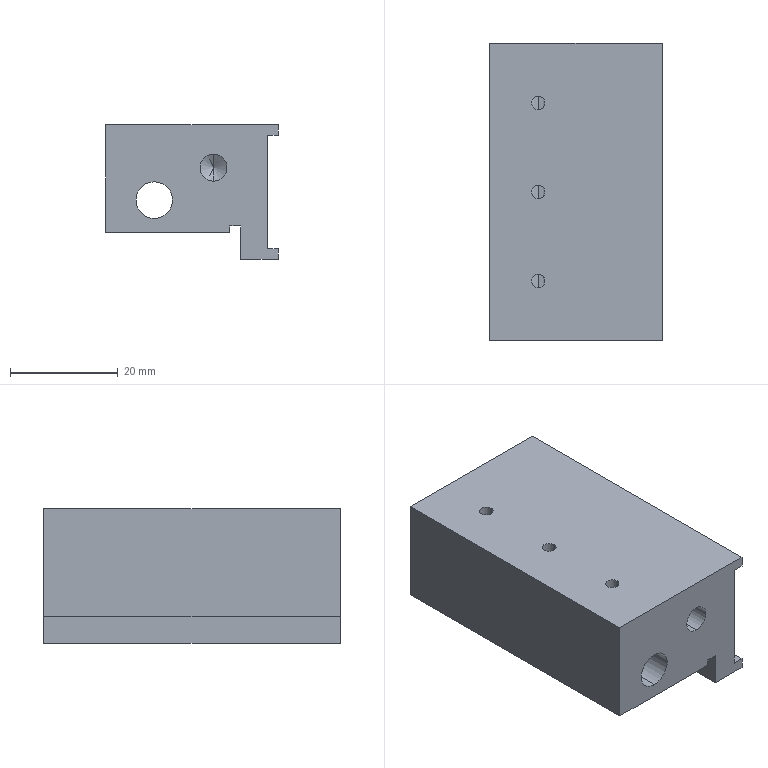Part | STEP file | 11-FG-B03311 | 1 solid | 44 faces | box 32 x 55 x 25 mm | volume 31224 mm3 | cylinder 20 | plane 16 | cone 8 | commonest cylinder face diameters 5 x8 2.5 x6 3.3 x4 6.8 x2
STEP:
#1=CARTESIAN_POINT('',(7.75,27.5,9.162));
#2=VERTEX_POINT('',#1);
#3=CARTESIAN_POINT('',(9.,26.25,9.4));
#4=VERTEX_POINT('',#3);
#5=CARTESIAN_POINT('',(7.75,27.5,9.162));
#6=CARTESIAN_POINT('',(7.75,27.336,9.162));
#7=CARTESIAN_POINT('',(7.783,27.17,9.176));
#8=CARTESIAN_POINT('',(7.909,26.868,9.221));
#9=CARTESIAN_POINT('',(8.001,26.732,9.252));
#10=CARTESIAN_POINT('',(8.232,26.501,9.314));
#11=CARTESIAN_POINT('',(8.368,26.409,9.344));
#12=CARTESIAN_POINT('',(8.595,26.315,9.377));
#13=CARTESIAN_POINT('',(8.673,26.291,9.385));
#14=CARTESIAN_POINT('',(8.834,26.258,9.397));
#15=CARTESIAN_POINT('',(8.918,26.25,9.4));
#16=CARTESIAN_POINT('',(9.,26.25,9.4));
#17=B_SPLINE_CURVE_WITH_KNOTS('',3,(#5,#6,#7,#8,#9,#10,#11,#12,#13,#14,#15,#16),.UNSPECIFIED.,.F.,.F.,(4,2,2,2,2,4),(0.003943,0.004435,0.004928,0.005421,0.005667,0.005913),.UNSPECIFIED.);
#18=EDGE_CURVE('',#2,#4,#17,.T.);
#19=ORIENTED_EDGE('',*,*,#18,.F.);
#20=CARTESIAN_POINT('',(7.75,27.5,20.));
#21=VERTEX_POINT('',#20);
#22=CARTESIAN_POINT('',(7.75,27.5,20.));
#23=DIRECTION('',(0.,0.,1.));
#24=VECTOR('',#23,1000.);
#25=LINE('',#22,#24);
#26=EDGE_CURVE('',#2,#21,#25,.T.);
#27=ORIENTED_EDGE('',*,*,#26,.T.);
#28=CARTESIAN_POINT('',(10.25,27.5,20.));
#29=VERTEX_POINT('',#28);
#30=CARTESIAN_POINT('',(9.,27.5,20.));
#31=DIRECTION('',(0.,0.,1.));
#32=DIRECTION('',(1.,0.,0.));
#33=AXIS2_PLACEMENT_3D('',#30,#31,#32);
#34=CIRCLE('',#33,1.25);
#35=EDGE_CURVE('',#21,#29,#34,.T.);
#36=ORIENTED_EDGE('',*,*,#35,.T.);
#37=CARTESIAN_POINT('',(10.25,27.5,9.162));
#38=VERTEX_POINT('',#37);
#39=CARTESIAN_POINT('',(10.25,27.5,20.));
#40=DIRECTION('',(0.,0.,1.));
#41=VECTOR('',#40,1000.);
#42=LINE('',#39,#41);
#43=EDGE_CURVE('',#38,#29,#42,.T.);
#44=ORIENTED_EDGE('',*,*,#43,.F.);
#45=CARTESIAN_POINT('',(9.,26.25,9.4));
#46=CARTESIAN_POINT('',(9.165,26.25,9.4));
#47=CARTESIAN_POINT('',(9.33,26.283,9.387));
#48=CARTESIAN_POINT('',(9.632,26.409,9.344));
#49=CARTESIAN_POINT('',(9.77,26.502,9.314));
#50=CARTESIAN_POINT('',(9.999,26.731,9.252));
#51=CARTESIAN_POINT('',(10.091,26.868,9.221));
#52=CARTESIAN_POINT('',(10.217,27.171,9.175));
#53=CARTESIAN_POINT('',(10.25,27.333,9.162));
#54=CARTESIAN_POINT('',(10.25,27.5,9.162));
#55=B_SPLINE_CURVE_WITH_KNOTS('',3,(#45,#46,#47,#48,#49,#50,#51,#52,#53,#54),.UNSPECIFIED.,.F.,.F.,(4,2,2,2,4),(0.005913,0.006406,0.006899,0.007392,0.007885),.UNSPECIFIED.);
#56=EDGE_CURVE('',#4,#38,#55,.T.);
#57=ORIENTED_EDGE('',*,*,#56,.F.);
#58=EDGE_LOOP('',(#19,#27,#36,#44,#57));
#59=FACE_OUTER_BOUND('',#58,.T.);
#60=CARTESIAN_POINT('',(9.,27.5,20.));
#61=DIRECTION('',(0.,0.,1.));
#62=DIRECTION('',(1.,0.,0.));
#63=AXIS2_PLACEMENT_3D('',#60,#61,#62);
#64=CYLINDRICAL_SURFACE('',#63,1.25);
#65=ADVANCED_FACE('',(#59),#64,.F.);
#66=CARTESIAN_POINT('',(7.75,44.,9.162));
#67=VERTEX_POINT('',#66);
#68=CARTESIAN_POINT('',(9.,42.75,9.4));
#69=VERTEX_POINT('',#68);
#70=CARTESIAN_POINT('',(7.75,44.,9.162));
#71=CARTESIAN_POINT('',(7.75,43.836,9.162));
#72=CARTESIAN_POINT('',(7.783,43.67,9.176));
#73=CARTESIAN_POINT('',(7.909,43.368,9.221));
#74=CARTESIAN_POINT('',(8.001,43.232,9.252));
#75=CARTESIAN_POINT('',(8.232,43.001,9.314));
#76=CARTESIAN_POINT('',(8.368,42.909,9.344));
#77=CARTESIAN_POINT('',(8.595,42.815,9.377));
#78=CARTESIAN_POINT('',(8.673,42.791,9.385));
#79=CARTESIAN_POINT('',(8.834,42.758,9.397));
#80=CARTESIAN_POINT('',(8.918,42.75,9.4));
#81=CARTESIAN_POINT('',(9.,42.75,9.4));
#82=B_SPLINE_CURVE_WITH_KNOTS('',3,(#70,#71,#72,#73,#74,#75,#76,#77,#78,#79,#80,#81),.UNSPECIFIED.,.F.,.F.,(4,2,2,2,2,4),(0.003943,0.004435,0.004928,0.005421,0.005667,0.005913),.UNSPECIFIED.);
#83=EDGE_CURVE('',#67,#69,#82,.T.);
#84=ORIENTED_EDGE('',*,*,#83,.F.);
#85=CARTESIAN_POINT('',(7.75,44.,20.));
#86=VERTEX_POINT('',#85);
#87=CARTESIAN_POINT('',(7.75,44.,20.));
#88=DIRECTION('',(0.,0.,1.));
#89=VECTOR('',#88,1000.);
#90=LINE('',#87,#89);
#91=EDGE_CURVE('',#67,#86,#90,.T.);
#92=ORIENTED_EDGE('',*,*,#91,.T.);
#93=CARTESIAN_POINT('',(10.25,44.,20.));
#94=VERTEX_POINT('',#93);
#95=CARTESIAN_POINT('',(9.,44.,20.));
#96=DIRECTION('',(0.,0.,1.));
#97=DIRECTION('',(1.,0.,0.));
#98=AXIS2_PLACEMENT_3D('',#95,#96,#97);
#99=CIRCLE('',#98,1.25);
#100=EDGE_CURVE('',#86,#94,#99,.T.);
#101=ORIENTED_EDGE('',*,*,#100,.T.);
#102=CARTESIAN_POINT('',(10.25,44.,9.162));
#103=VERTEX_POINT('',#102);
#104=CARTESIAN_POINT('',(10.25,44.,20.));
#105=DIRECTION('',(0.,0.,1.));
#106=VECTOR('',#105,1000.);
#107=LINE('',#104,#106);
#108=EDGE_CURVE('',#103,#94,#107,.T.);
#109=ORIENTED_EDGE('',*,*,#108,.F.);
#110=CARTESIAN_POINT('',(9.,42.75,9.4));
#111=CARTESIAN_POINT('',(9.165,42.75,9.4));
#112=CARTESIAN_POINT('',(9.33,42.783,9.387));
#113=CARTESIAN_POINT('',(9.632,42.909,9.344));
#114=CARTESIAN_POINT('',(9.77,43.002,9.314));
#115=CARTESIAN_POINT('',(9.999,43.231,9.252));
#116=CARTESIAN_POINT('',(10.091,43.368,9.221));
#117=CARTESIAN_POINT('',(10.217,43.671,9.175));
#118=CARTESIAN_POINT('',(10.25,43.833,9.162));
#119=CARTESIAN_POINT('',(10.25,44.,9.162));
#120=B_SPLINE_CURVE_WITH_KNOTS('',3,(#110,#111,#112,#113,#114,#115,#116,#117,#118,#119),.UNSPECIFIED.,.F.,.F.,(4,2,2,2,4),(0.005913,0.006406,0.006899,0.007392,0.007885),.UNSPECIFIED.);
#121=EDGE_CURVE('',#69,#103,#120,.T.);
#122=ORIENTED_EDGE('',*,*,#121,.F.);
#123=EDGE_LOOP('',(#84,#92,#101,#109,#122));
#124=FACE_OUTER_BOUND('',#123,.T.);
#125=CARTESIAN_POINT('',(9.,44.,20.));
#126=DIRECTION('',(0.,0.,1.));
#127=DIRECTION('',(1.,0.,0.));
#128=AXIS2_PLACEMENT_3D('',#125,#126,#127);
#129=CYLINDRICAL_SURFACE('',#128,1.25);
#130=ADVANCED_FACE('',(#124),#129,.F.);
#131=CARTESIAN_POINT('',(7.75,11.,9.162));
#132=VERTEX_POINT('',#131);
#133=CARTESIAN_POINT('',(9.,9.75,9.4));
#134=VERTEX_POINT('',#133);
#135=CARTESIAN_POINT('',(7.75,11.,9.162));
#136=CARTESIAN_POINT('',(7.75,10.836,9.162));
#137=CARTESIAN_POINT('',(7.783,10.67,9.176));
#138=CARTESIAN_POINT('',(7.909,10.368,9.221));
#139=CARTESIAN_POINT('',(8.001,10.232,9.252));
#140=CARTESIAN_POINT('',(8.232,10.001,9.314));
#141=CARTESIAN_POINT('',(8.368,9.909,9.344));
#142=CARTESIAN_POINT('',(8.595,9.815,9.377));
#143=CARTESIAN_POINT('',(8.673,9.791,9.385));
#144=CARTESIAN_POINT('',(8.834,9.758,9.397));
#145=CARTESIAN_POINT('',(8.918,9.75,9.4));
#146=CARTESIAN_POINT('',(9.,9.75,9.4));
#147=B_SPLINE_CURVE_WITH_KNOTS('',3,(#135,#136,#137,#138,#139,#140,#141,#142,#143,#144,#145,#146),.UNSPECIFIED.,.F.,.F.,(4,2,2,2,2,4),(0.003943,0.004435,0.004928,0.005421,0.005667,0.005913),.UNSPECIFIED.);
#148=EDGE_CURVE('',#132,#134,#147,.T.);
#149=ORIENTED_EDGE('',*,*,#148,.F.);
#150=CARTESIAN_POINT('',(7.75,11.,20.));
#151=VERTEX_POINT('',#150);
#152=CARTESIAN_POINT('',(7.75,11.,20.));
#153=DIRECTION('',(0.,0.,1.));
#154=VECTOR('',#153,1000.);
#155=LINE('',#152,#154);
#156=EDGE_CURVE('',#132,#151,#155,.T.);
#157=ORIENTED_EDGE('',*,*,#156,.T.);
#158=CARTESIAN_POINT('',(10.25,11.,20.));
#159=VERTEX_POINT('',#158);
#160=CARTESIAN_POINT('',(9.,11.,20.));
#161=DIRECTION('',(0.,0.,1.));
#162=DIRECTION('',(1.,0.,0.));
#163=AXIS2_PLACEMENT_3D('',#160,#161,#162);
#164=CIRCLE('',#163,1.25);
#165=EDGE_CURVE('',#151,#159,#164,.T.);
#166=ORIENTED_EDGE('',*,*,#165,.T.);
#167=CARTESIAN_POINT('',(10.25,11.,9.162));
#168=VERTEX_POINT('',#167);
#169=CARTESIAN_POINT('',(10.25,11.,20.));
#170=DIRECTION('',(0.,0.,1.));
#171=VECTOR('',#170,1000.);
#172=LINE('',#169,#171);
#173=EDGE_CURVE('',#168,#159,#172,.T.);
#174=ORIENTED_EDGE('',*,*,#173,.F.);
#175=CARTESIAN_POINT('',(9.,9.75,9.4));
#176=CARTESIAN_POINT('',(9.165,9.75,9.4));
#177=CARTESIAN_POINT('',(9.33,9.783,9.387));
#178=CARTESIAN_POINT('',(9.632,9.909,9.344));
#179=CARTESIAN_POINT('',(9.77,10.002,9.314));
#180=CARTESIAN_POINT('',(9.999,10.231,9.252));
#181=CARTESIAN_POINT('',(10.091,10.368,9.221));
#182=CARTESIAN_POINT('',(10.217,10.671,9.175));
#183=CARTESIAN_POINT('',(10.25,10.833,9.162));
#184=CARTESIAN_POINT('',(10.25,11.,9.162));
#185=B_SPLINE_CURVE_WITH_KNOTS('',3,(#175,#176,#177,#178,#179,#180,#181,#182,#183,#184),.UNSPECIFIED.,.F.,.F.,(4,2,2,2,4),(0.005913,0.006406,0.006899,0.007392,0.007885),.UNSPECIFIED.);
#186=EDGE_CURVE('',#134,#168,#185,.T.);
#187=ORIENTED_EDGE('',*,*,#186,.F.);
#188=EDGE_LOOP('',(#149,#157,#166,#174,#187));
#189=FACE_OUTER_BOUND('',#188,.T.);
#190=CARTESIAN_POINT('',(9.,11.,20.));
#191=DIRECTION('',(0.,0.,1.));
#192=DIRECTION('',(1.,0.,0.));
#193=AXIS2_PLACEMENT_3D('',#190,#191,#192);
#194=CYLINDRICAL_SURFACE('',#193,1.25);
#195=ADVANCED_FACE('',(#189),#194,.F.);
#196=CARTESIAN_POINT('',(20.,40.,9.5));
#197=VERTEX_POINT('',#196);
#198=CARTESIAN_POINT('',(20.,40.,14.5));
#199=VERTEX_POINT('',#198);
#200=CARTESIAN_POINT('',(20.,40.,12.));
#201=DIRECTION('',(0.,1.,0.));
#202=DIRECTION('',(0.,0.,1.));
#203=AXIS2_PLACEMENT_3D('',#200,#201,#202);
#204=CIRCLE('',#203,2.5);
#205=EDGE_CURVE('',#197,#199,#204,.T.);
#206=ORIENTED_EDGE('',*,*,#205,.F.);
#207=CARTESIAN_POINT('',(20.,55.,9.5));
#208=VERTEX_POINT('',#207);
#209=CARTESIAN_POINT('',(20.,55.,9.5));
#210=DIRECTION('',(0.,1.,0.));
#211=VECTOR('',#210,1000.);
#212=LINE('',#209,#211);
#213=EDGE_CURVE('',#197,#208,#212,.T.);
#214=ORIENTED_EDGE('',*,*,#213,.T.);
#215=CARTESIAN_POINT('',(20.,55.,14.5));
#216=VERTEX_POINT('',#215);
#217=CARTESIAN_POINT('',(20.,55.,12.));
#218=DIRECTION('',(0.,1.,0.));
#219=DIRECTION('',(0.,0.,1.));
#220=AXIS2_PLACEMENT_3D('',#217,#218,#219);
#221=CIRCLE('',#220,2.5);
#222=EDGE_CURVE('',#208,#216,#221,.T.);
#223=ORIENTED_EDGE('',*,*,#222,.T.);
#224=CARTESIAN_POINT('',(20.,55.,14.5));
#225=DIRECTION('',(0.,1.,0.));
#226=VECTOR('',#225,1000.);
#227=LINE('',#224,#226);
#228=EDGE_CURVE('',#199,#216,#227,.T.);
#229=ORIENTED_EDGE('',*,*,#228,.F.);
#230=EDGE_LOOP('',(#206,#214,#223,#229));
#231=FACE_OUTER_BOUND('',#230,.T.);
#232=CARTESIAN_POINT('',(20.,55.,12.));
#233=DIRECTION('',(0.,1.,0.));
#234=DIRECTION('',(0.,0.,1.));
#235=AXIS2_PLACEMENT_3D('',#232,#233,#234);
#236=CYLINDRICAL_SURFACE('',#235,2.5);
#237=ADVANCED_FACE('',(#231),#236,.F.);
#238=CARTESIAN_POINT('',(20.,38.498,12.));
#239=VERTEX_POINT('',#238);
#240=CARTESIAN_POINT('',(20.,40.,14.5));
#241=DIRECTION('',(0.,0.515,0.8572));
#242=VECTOR('',#241,1000.);
#243=LINE('',#240,#242);
#244=EDGE_CURVE('',#239,#199,#243,.T.);
#245=ORIENTED_EDGE('',*,*,#244,.F.);
#246=CARTESIAN_POINT('',(20.,40.,9.5));
#247=DIRECTION('',(0.,0.515,-0.8572));
#248=VECTOR('',#247,1000.);
#249=LINE('',#246,#248);
#250=EDGE_CURVE('',#239,#197,#249,.T.);
#251=ORIENTED_EDGE('',*,*,#250,.T.);
#252=ORIENTED_EDGE('',*,*,#205,.T.);
#253=EDGE_LOOP('',(#245,#251,#252));
#254=FACE_OUTER_BOUND('',#253,.T.);
#255=CARTESIAN_POINT('',(20.,40.,12.));
#256=DIRECTION('',(0.,1.,0.));
#257=DIRECTION('',(0.,0.,1.));
#258=AXIS2_PLACEMENT_3D('',#255,#256,#257);
#259=CONICAL_SURFACE('',#258,2.5,1.03);
#260=ADVANCED_FACE('',(#254),#259,.F.);
#261=CARTESIAN_POINT('',(18.,48.5,9.));
#262=VERTEX_POINT('',#261);
#263=CARTESIAN_POINT('',(18.,48.5,4.));
#264=VERTEX_POINT('',#263);
#265=CARTESIAN_POINT('',(18.,48.5,6.5));
#266=DIRECTION('',(1.,0.,0.));
#267=DIRECTION('',(0.,0.,-1.));
#268=AXIS2_PLACEMENT_3D('',#265,#266,#267);
#269=CIRCLE('',#268,2.5);
#270=EDGE_CURVE('',#262,#264,#269,.T.);
#271=ORIENTED_EDGE('',*,*,#270,.F.);
#272=CARTESIAN_POINT('',(30.,48.5,9.));
#273=VERTEX_POINT('',#272);
#274=CARTESIAN_POINT('',(30.,48.5,9.));
#275=DIRECTION('',(1.,0.,0.));
#276=VECTOR('',#275,1000.);
#277=LINE('',#274,#276);
#278=EDGE_CURVE('',#262,#273,#277,.T.);
#279=ORIENTED_EDGE('',*,*,#278,.T.);
#280=CARTESIAN_POINT('',(30.,48.5,4.));
#281=VERTEX_POINT('',#280);
#282=CARTESIAN_POINT('',(30.,48.5,6.5));
#283=DIRECTION('',(1.,0.,0.));
#284=DIRECTION('',(0.,0.,-1.));
#285=AXIS2_PLACEMENT_3D('',#282,#283,#284);
#286=CIRCLE('',#285,2.5);
#287=EDGE_CURVE('',#273,#281,#286,.T.);
#288=ORIENTED_EDGE('',*,*,#287,.T.);
#289=CARTESIAN_POINT('',(30.,48.5,4.));
#290=DIRECTION('',(1.,0.,0.));
#291=VECTOR('',#290,1000.);
#292=LINE('',#289,#291);
#293=EDGE_CURVE('',#264,#281,#292,.T.);
#294=ORIENTED_EDGE('',*,*,#293,.F.);
#295=EDGE_LOOP('',(#271,#279,#288,#294));
#296=FACE_OUTER_BOUND('',#295,.T.);
#297=CARTESIAN_POINT('',(30.,48.5,6.5));
#298=DIRECTION('',(1.,0.,0.));
#299=DIRECTION('',(0.,0.,-1.));
#300=AXIS2_PLACEMENT_3D('',#297,#298,#299);
#301=CYLINDRICAL_SURFACE('',#300,2.5);
#302=ADVANCED_FACE('',(#296),#301,.F.);
#303=CARTESIAN_POINT('',(16.498,48.5,6.5));
#304=VERTEX_POINT('',#303);
#305=CARTESIAN_POINT('',(18.,48.5,4.));
#306=DIRECTION('',(0.515,0.,-0.8572));
#307=VECTOR('',#306,1000.);
#308=LINE('',#305,#307);
#309=EDGE_CURVE('',#304,#264,#308,.T.);
#310=ORIENTED_EDGE('',*,*,#309,.F.);
#311=CARTESIAN_POINT('',(18.,48.5,9.));
#312=DIRECTION('',(0.515,0.,0.8572));
#313=VECTOR('',#312,1000.);
#314=LINE('',#311,#313);
#315=EDGE_CURVE('',#304,#262,#314,.T.);
#316=ORIENTED_EDGE('',*,*,#315,.T.);
#317=ORIENTED_EDGE('',*,*,#270,.T.);
#318=EDGE_LOOP('',(#310,#316,#317));
#319=FACE_OUTER_BOUND('',#318,.T.);
#320=CARTESIAN_POINT('',(18.,48.5,6.5));
#321=DIRECTION('',(1.,0.,0.));
#322=DIRECTION('',(0.,0.,-1.));
#323=AXIS2_PLACEMENT_3D('',#320,#321,#322);
#324=CONICAL_SURFACE('',#323,2.5,1.03);
#325=ADVANCED_FACE('',(#319),#324,.F.);
#326=CARTESIAN_POINT('',(18.,6.5,9.));
#327=VERTEX_POINT('',#326);
#328=CARTESIAN_POINT('',(18.,6.5,4.));
#329=VERTEX_POINT('',#328);
#330=CARTESIAN_POINT('',(18.,6.5,6.5));
#331=DIRECTION('',(1.,0.,0.));
#332=DIRECTION('',(0.,0.,-1.));
#333=AXIS2_PLACEMENT_3D('',#330,#331,#332);
#334=CIRCLE('',#333,2.5);
#335=EDGE_CURVE('',#327,#329,#334,.T.);
#336=ORIENTED_EDGE('',*,*,#335,.F.);
#337=CARTESIAN_POINT('',(30.,6.5,9.));
#338=VERTEX_POINT('',#337);
#339=CARTESIAN_POINT('',(30.,6.5,9.));
#340=DIRECTION('',(1.,0.,0.));
#341=VECTOR('',#340,1000.);
#342=LINE('',#339,#341);
#343=EDGE_CURVE('',#327,#338,#342,.T.);
#344=ORIENTED_EDGE('',*,*,#343,.T.);
#345=CARTESIAN_POINT('',(30.,6.5,4.));
#346=VERTEX_POINT('',#345);
#347=CARTESIAN_POINT('',(30.,6.5,6.5));
#348=DIRECTION('',(1.,0.,0.));
#349=DIRECTION('',(0.,0.,-1.));
#350=AXIS2_PLACEMENT_3D('',#347,#348,#349);
#351=CIRCLE('',#350,2.5);
#352=EDGE_CURVE('',#338,#346,#351,.T.);
#353=ORIENTED_EDGE('',*,*,#352,.T.);
#354=CARTESIAN_POINT('',(30.,6.5,4.));
#355=DIRECTION('',(1.,0.,0.));
#356=VECTOR('',#355,1000.);
#357=LINE('',#354,#356);
#358=EDGE_CURVE('',#329,#346,#357,.T.);
#359=ORIENTED_EDGE('',*,*,#358,.F.);
#360=EDGE_LOOP('',(#336,#344,#353,#359));
#361=FACE_OUTER_BOUND('',#360,.T.);
#362=CARTESIAN_POINT('',(30.,6.5,6.5));
#363=DIRECTION('',(1.,0.,0.));
#364=DIRECTION('',(0.,0.,-1.));
#365=AXIS2_PLACEMENT_3D('',#362,#363,#364);
#366=CYLINDRICAL_SURFACE('',#365,2.5);
#367=ADVANCED_FACE('',(#361),#366,.F.);
#368=CARTESIAN_POINT('',(16.498,6.5,6.5));
#369=VERTEX_POINT('',#368);
#370=CARTESIAN_POINT('',(18.,6.5,4.));
#371=DIRECTION('',(0.515,0.,-0.8572));
#372=VECTOR('',#371,1000.);
#373=LINE('',#370,#372);
#374=EDGE_CURVE('',#369,#329,#373,.T.);
#375=ORIENTED_EDGE('',*,*,#374,.F.);
#376=CARTESIAN_POINT('',(18.,6.5,9.));
#377=DIRECTION('',(0.515,0.,0.8572));
#378=VECTOR('',#377,1000.);
#379=LINE('',#376,#378);
#380=EDGE_CURVE('',#369,#327,#379,.T.);
#381=ORIENTED_EDGE('',*,*,#380,.T.);
#382=ORIENTED_EDGE('',*,*,#335,.T.);
#383=EDGE_LOOP('',(#375,#381,#382));
#384=FACE_OUTER_BOUND('',#383,.T.);
#385=CARTESIAN_POINT('',(18.,6.5,6.5));
#386=DIRECTION('',(1.,0.,0.));
#387=DIRECTION('',(0.,0.,-1.));
#388=AXIS2_PLACEMENT_3D('',#385,#386,#387);
#389=CONICAL_SURFACE('',#388,2.5,1.03);
#390=ADVANCED_FACE('',(#384),#389,.F.);
#391=CARTESIAN_POINT('',(20.,15.,14.5));
#392=VERTEX_POINT('',#391);
#393=CARTESIAN_POINT('',(20.,15.,9.5));
#394=VERTEX_POINT('',#393);
#395=CARTESIAN_POINT('',(20.,15.,12.));
#396=DIRECTION('',(0.,-1.,0.));
#397=DIRECTION('',(0.,0.,-1.));
#398=AXIS2_PLACEMENT_3D('',#395,#396,#397);
#399=CIRCLE('',#398,2.5);
#400=EDGE_CURVE('',#392,#394,#399,.T.);
#401=ORIENTED_EDGE('',*,*,#400,.F.);
#402=CARTESIAN_POINT('',(20.,0.,14.5));
#403=VERTEX_POINT('',#402);
#404=CARTESIAN_POINT('',(20.,0.,14.5));
#405=DIRECTION('',(0.,-1.,0.));
#406=VECTOR('',#405,1000.);
#407=LINE('',#404,#406);
#408=EDGE_CURVE('',#392,#403,#407,.T.);
#409=ORIENTED_EDGE('',*,*,#408,.T.);
#410=CARTESIAN_POINT('',(20.,0.,9.5));
#411=VERTEX_POINT('',#410);
#412=CARTESIAN_POINT('',(20.,0.,12.));
#413=DIRECTION('',(0.,-1.,0.));
#414=DIRECTION('',(0.,0.,-1.));
#415=AXIS2_PLACEMENT_3D('',#412,#413,#414);
#416=CIRCLE('',#415,2.5);
#417=EDGE_CURVE('',#403,#411,#416,.T.);
#418=ORIENTED_EDGE('',*,*,#417,.T.);
#419=CARTESIAN_POINT('',(20.,0.,9.5));
#420=DIRECTION('',(0.,-1.,0.));
#421=VECTOR('',#420,1000.);
#422=LINE('',#419,#421);
#423=EDGE_CURVE('',#394,#411,#422,.T.);
#424=ORIENTED_EDGE('',*,*,#423,.F.);
#425=EDGE_LOOP('',(#401,#409,#418,#424));
#426=FACE_OUTER_BOUND('',#425,.T.);
#427=CARTESIAN_POINT('',(20.,0.,12.));
#428=DIRECTION('',(0.,-1.,0.));
#429=DIRECTION('',(0.,0.,-1.));
#430=AXIS2_PLACEMENT_3D('',#427,#428,#429);
#431=CYLINDRICAL_SURFACE('',#430,2.5);
#432=ADVANCED_FACE('',(#426),#431,.F.);
#433=CARTESIAN_POINT('',(20.,16.502,12.));
#434=VERTEX_POINT('',#433);
#435=CARTESIAN_POINT('',(20.,15.,9.5));
#436=DIRECTION('',(0.,-0.515,-0.8572));
#437=VECTOR('',#436,1000.);
#438=LINE('',#435,#437);
#439=EDGE_CURVE('',#434,#394,#438,.T.);
#440=ORIENTED_EDGE('',*,*,#439,.F.);
#441=CARTESIAN_POINT('',(20.,15.,14.5));
#442=DIRECTION('',(0.,-0.515,0.8572));
#443=VECTOR('',#442,1000.);
#444=LINE('',#441,#443);
#445=EDGE_CURVE('',#434,#392,#444,.T.);
#446=ORIENTED_EDGE('',*,*,#445,.T.);
#447=ORIENTED_EDGE('',*,*,#400,.T.);
#448=EDGE_LOOP('',(#440,#446,#447));
#449=FACE_OUTER_BOUND('',#448,.T.);
#450=CARTESIAN_POINT('',(20.,15.,12.));
#451=DIRECTION('',(0.,-1.,0.));
#452=DIRECTION('',(0.,0.,-1.));
#453=AXIS2_PLACEMENT_3D('',#450,#451,#452);
#454=CONICAL_SURFACE('',#453,2.5,1.03);
#455=ADVANCED_FACE('',(#449),#454,.F.);
#456=CARTESIAN_POINT('',(16.65,45.,12.));
#457=VERTEX_POINT('',#456);
#458=CARTESIAN_POINT('',(13.35,45.,12.));
#459=VERTEX_POINT('',#458);
#460=CARTESIAN_POINT('',(15.,45.,12.));
#461=DIRECTION('',(0.,0.,-1.));
#462=DIRECTION('',(-1.,0.,0.));
#463=AXIS2_PLACEMENT_3D('',#460,#461,#462);
#464=CIRCLE('',#463,1.65);
#465=EDGE_CURVE('',#457,#459,#464,.T.);
#466=ORIENTED_EDGE('',*,*,#465,.F.);
#467=CARTESIAN_POINT('',(16.65,45.,0.));
#468=VERTEX_POINT('',#467);
#469=CARTESIAN_POINT('',(16.65,45.,0.));
#470=DIRECTION('',(0.,0.,-1.));
#471=VECTOR('',#470,1000.);
#472=LINE('',#469,#471);
#473=EDGE_CURVE('',#457,#468,#472,.T.);
#474=ORIENTED_EDGE('',*,*,#473,.T.);
#475=CARTESIAN_POINT('',(13.35,45.,0.));
#476=VERTEX_POINT('',#475);
#477=CARTESIAN_POINT('',(15.,45.,0.));
#478=DIRECTION('',(0.,0.,-1.));
#479=DIRECTION('',(-1.,0.,0.));
#480=AXIS2_PLACEMENT_3D('',#477,#478,#479);
#481=CIRCLE('',#480,1.65);
#482=EDGE_CURVE('',#468,#476,#481,.T.);
#483=ORIENTED_EDGE('',*,*,#482,.T.);
#484=CARTESIAN_POINT('',(13.35,45.,0.));
#485=DIRECTION('',(0.,0.,-1.));
#486=VECTOR('',#485,1000.);
#487=LINE('',#484,#486);
#488=EDGE_CURVE('',#459,#476,#487,.T.);
#489=ORIENTED_EDGE('',*,*,#488,.F.);
#490=EDGE_LOOP('',(#466,#474,#483,#489));
#491=FACE_OUTER_BOUND('',#490,.T.);
#492=CARTESIAN_POINT('',(15.,45.,0.));
#493=DIRECTION('',(0.,0.,-1.));
#494=DIRECTION('',(-1.,0.,0.));
#495=AXIS2_PLACEMENT_3D('',#492,#493,#494);
#496=CYLINDRICAL_SURFACE('',#495,1.65);
#497=ADVANCED_FACE('',(#491),#496,.F.);
#498=CARTESIAN_POINT('',(16.65,10.,12.));
#499=VERTEX_POINT('',#498);
#500=CARTESIAN_POINT('',(13.35,10.,12.));
#501=VERTEX_POINT('',#500);
#502=CARTESIAN_POINT('',(15.,10.,12.));
#503=DIRECTION('',(0.,0.,-1.));
#504=DIRECTION('',(-1.,0.,0.));
#505=AXIS2_PLACEMENT_3D('',#502,#503,#504);
#506=CIRCLE('',#505,1.65);
#507=EDGE_CURVE('',#499,#501,#506,.T.);
#508=ORIENTED_EDGE('',*,*,#507,.F.);
#509=CARTESIAN_POINT('',(16.65,10.,0.));
#510=VERTEX_POINT('',#509);
#511=CARTESIAN_POINT('',(16.65,10.,0.));
#512=DIRECTION('',(0.,0.,-1.));
#513=VECTOR('',#512,1000.);
#514=LINE('',#511,#513);
#515=EDGE_CURVE('',#499,#510,#514,.T.);
#516=ORIENTED_EDGE('',*,*,#515,.T.);
#517=CARTESIAN_POINT('',(13.35,10.,0.));
#518=VERTEX_POINT('',#517);
#519=CARTESIAN_POINT('',(15.,10.,0.));
#520=DIRECTION('',(0.,0.,-1.));
#521=DIRECTION('',(-1.,0.,0.));
#522=AXIS2_PLACEMENT_3D('',#519,#520,#521);
#523=CIRCLE('',#522,1.65);
#524=EDGE_CURVE('',#510,#518,#523,.T.);
#525=ORIENTED_EDGE('',*,*,#524,.T.);
#526=CARTESIAN_POINT('',(13.35,10.,0.));
#527=DIRECTION('',(0.,0.,-1.));
#528=VECTOR('',#527,1000.);
#529=LINE('',#526,#528);
#530=EDGE_CURVE('',#501,#518,#529,.T.);
#531=ORIENTED_EDGE('',*,*,#530,.F.);
#532=EDGE_LOOP('',(#508,#516,#525,#531));
#533=FACE_OUTER_BOUND('',#532,.T.);
#534=CARTESIAN_POINT('',(15.,10.,0.));
#535=DIRECTION('',(0.,0.,-1.));
#536=DIRECTION('',(-1.,0.,0.));
#537=AXIS2_PLACEMENT_3D('',#534,#535,#536);
#538=CYLINDRICAL_SURFACE('',#537,1.65);
#539=ADVANCED_FACE('',(#533),#538,.F.);
#540=CARTESIAN_POINT('',(9.,55.,9.4));
#541=VERTEX_POINT('',#540);
#542=CARTESIAN_POINT('',(9.,55.,2.6));
#543=VERTEX_POINT('',#542);
#544=CARTESIAN_POINT('',(9.,55.,6.));
#545=DIRECTION('',(0.,-1.,0.));
#546=DIRECTION('',(0.,0.,-1.));
#547=AXIS2_PLACEMENT_3D('',#544,#545,#546);
#548=CIRCLE('',#547,3.4);
#549=EDGE_CURVE('',#541,#543,#548,.T.);
#550=ORIENTED_EDGE('',*,*,#549,.F.);
#551=CARTESIAN_POINT('',(9.,45.25,9.4));
#552=VERTEX_POINT('',#551);
#553=CARTESIAN_POINT('',(9.,55.,9.4));
#554=DIRECTION('',(0.,-1.,0.));
#555=VECTOR('',#554,1000.);
#556=LINE('',#553,#555);
#557=EDGE_CURVE('',#541,#552,#556,.T.);
#558=ORIENTED_EDGE('',*,*,#557,.T.);
#559=CARTESIAN_POINT('',(9.,45.25,9.4));
#560=CARTESIAN_POINT('',(8.918,45.25,9.4));
#561=CARTESIAN_POINT('',(8.834,45.242,9.397));
#562=CARTESIAN_POINT('',(8.673,45.209,9.385));
#563=CARTESIAN_POINT('',(8.595,45.185,9.377));
#564=CARTESIAN_POINT('',(8.366,45.09,9.344));
#565=CARTESIAN_POINT('',(8.23,44.998,9.314));
#566=CARTESIAN_POINT('',(8.001,44.768,9.252));
#567=CARTESIAN_POINT('',(7.908,44.63,9.221));
#568=CARTESIAN_POINT('',(7.783,44.33,9.176));
#569=CARTESIAN_POINT('',(7.75,44.164,9.162));
#570=CARTESIAN_POINT('',(7.75,44.,9.162));
#571=B_SPLINE_CURVE_WITH_KNOTS('',3,(#559,#560,#561,#562,#563,#564,#565,#566,#567,#568,#569,#570),.UNSPECIFIED.,.F.,.F.,(4,2,2,2,2,4),(0.001972,0.002218,0.002465,0.002957,0.00345,0.003943),.UNSPECIFIED.);
#572=EDGE_CURVE('',#552,#67,#571,.T.);
#573=ORIENTED_EDGE('',*,*,#572,.T.);
#574=ORIENTED_EDGE('',*,*,#83,.T.);
#575=CARTESIAN_POINT('',(9.,28.75,9.4));
#576=VERTEX_POINT('',#575);
#577=CARTESIAN_POINT('',(9.,55.,9.4));
#578=DIRECTION('',(0.,-1.,0.));
#579=VECTOR('',#578,1000.);
#580=LINE('',#577,#579);
#581=EDGE_CURVE('',#69,#576,#580,.T.);
#582=ORIENTED_EDGE('',*,*,#581,.T.);
#583=CARTESIAN_POINT('',(9.,28.75,9.4));
#584=CARTESIAN_POINT('',(8.918,28.75,9.4));
#585=CARTESIAN_POINT('',(8.834,28.742,9.397));
#586=CARTESIAN_POINT('',(8.673,28.709,9.385));
#587=CARTESIAN_POINT('',(8.595,28.685,9.377));
#588=CARTESIAN_POINT('',(8.366,28.59,9.344));
#589=CARTESIAN_POINT('',(8.23,28.498,9.314));
#590=CARTESIAN_POINT('',(8.001,28.268,9.252));
#591=CARTESIAN_POINT('',(7.908,28.13,9.221));
#592=CARTESIAN_POINT('',(7.783,27.83,9.176));
#593=CARTESIAN_POINT('',(7.75,27.664,9.162));
#594=CARTESIAN_POINT('',(7.75,27.5,9.162));
#595=B_SPLINE_CURVE_WITH_KNOTS('',3,(#583,#584,#585,#586,#587,#588,#589,#590,#591,#592,#593,#594),.UNSPECIFIED.,.F.,.F.,(4,2,2,2,2,4),(0.001972,0.002218,0.002465,0.002957,0.00345,0.003943),.UNSPECIFIED.);
#596=EDGE_CURVE('',#576,#2,#595,.T.);
#597=ORIENTED_EDGE('',*,*,#596,.T.);
#598=ORIENTED_EDGE('',*,*,#18,.T.);
#599=CARTESIAN_POINT('',(9.,12.25,9.4));
#600=VERTEX_POINT('',#599);
#601=CARTESIAN_POINT('',(9.,55.,9.4));
#602=DIRECTION('',(0.,-1.,0.));
#603=VECTOR('',#602,1000.);
#604=LINE('',#601,#603);
#605=EDGE_CURVE('',#4,#600,#604,.T.);
#606=ORIENTED_EDGE('',*,*,#605,.T.);
#607=CARTESIAN_POINT('',(9.,12.25,9.4));
#608=CARTESIAN_POINT('',(8.918,12.25,9.4));
#609=CARTESIAN_POINT('',(8.834,12.242,9.397));
#610=CARTESIAN_POINT('',(8.673,12.209,9.385));
#611=CARTESIAN_POINT('',(8.595,12.185,9.377));
#612=CARTESIAN_POINT('',(8.366,12.09,9.344));
#613=CARTESIAN_POINT('',(8.23,11.998,9.314));
#614=CARTESIAN_POINT('',(8.001,11.768,9.252));
#615=CARTESIAN_POINT('',(7.908,11.63,9.221));
#616=CARTESIAN_POINT('',(7.783,11.33,9.176));
#617=CARTESIAN_POINT('',(7.75,11.164,9.162));
#618=CARTESIAN_POINT('',(7.75,11.,9.162));
#619=B_SPLINE_CURVE_WITH_KNOTS('',3,(#607,#608,#609,#610,#611,#612,#613,#614,#615,#616,#617,#618),.UNSPECIFIED.,.F.,.F.,(4,2,2,2,2,4),(0.001972,0.002218,0.002465,0.002957,0.00345,0.003943),.UNSPECIFIED.);
#620=EDGE_CURVE('',#600,#132,#619,.T.);
#621=ORIENTED_EDGE('',*,*,#620,.T.);
#622=ORIENTED_EDGE('',*,*,#148,.T.);
#623=CARTESIAN_POINT('',(9.,0.,9.4));
#624=VERTEX_POINT('',#623);
#625=CARTESIAN_POINT('',(9.,55.,9.4));
#626=DIRECTION('',(0.,-1.,0.));
#627=VECTOR('',#626,1000.);
#628=LINE('',#625,#627);
#629=EDGE_CURVE('',#134,#624,#628,.T.);
#630=ORIENTED_EDGE('',*,*,#629,.T.);
#631=CARTESIAN_POINT('',(9.,0.,2.6));
#632=VERTEX_POINT('',#631);
#633=CARTESIAN_POINT('',(9.,0.,6.));
#634=DIRECTION('',(0.,-1.,0.));
#635=DIRECTION('',(0.,0.,-1.));
#636=AXIS2_PLACEMENT_3D('',#633,#634,#635);
#637=CIRCLE('',#636,3.4);
#638=EDGE_CURVE('',#624,#632,#637,.T.);
#639=ORIENTED_EDGE('',*,*,#638,.T.);
#640=CARTESIAN_POINT('',(9.,55.,2.6));
#641=DIRECTION('',(0.,-1.,0.));
#642=VECTOR('',#641,1000.);
#643=LINE('',#640,#642);
#644=EDGE_CURVE('',#543,#632,#643,.T.);
#645=ORIENTED_EDGE('',*,*,#644,.F.);
#646=EDGE_LOOP('',(#550,#558,#573,#574,#582,#597,#598,#606,#621,#622,#630,#639,#645));
#647=FACE_OUTER_BOUND('',#646,.T.);
#648=CARTESIAN_POINT('',(9.,55.,6.));
#649=DIRECTION('',(0.,-1.,0.));
#650=DIRECTION('',(0.,0.,-1.));
#651=AXIS2_PLACEMENT_3D('',#648,#649,#650);
#652=CYLINDRICAL_SURFACE('',#651,3.4);
#653=ADVANCED_FACE('',(#647),#652,.F.);
#654=CARTESIAN_POINT('',(15.,45.,0.));
#655=DIRECTION('',(0.,0.,-1.));
#656=DIRECTION('',(-1.,0.,0.));
#657=AXIS2_PLACEMENT_3D('',#654,#655,#656);
#658=CIRCLE('',#657,1.65);
#659=EDGE_CURVE('',#476,#468,#658,.T.);
#660=ORIENTED_EDGE('',*,*,#659,.F.);
#661=ORIENTED_EDGE('',*,*,#482,.F.);
#662=EDGE_LOOP('',(#660,#661));
#663=FACE_BOUND('',#662,.T.);
#664=CARTESIAN_POINT('',(15.,10.,0.));
#665=DIRECTION('',(0.,0.,-1.));
#666=DIRECTION('',(-1.,0.,0.));
#667=AXIS2_PLACEMENT_3D('',#664,#665,#666);
#668=CIRCLE('',#667,1.65);
#669=EDGE_CURVE('',#518,#510,#668,.T.);
#670=ORIENTED_EDGE('',*,*,#669,.F.);
#671=ORIENTED_EDGE('',*,*,#524,.F.);
#672=EDGE_LOOP('',(#670,#671));
#673=FACE_BOUND('',#672,.T.);
#674=CARTESIAN_POINT('',(23.,0.,0.));
#675=VERTEX_POINT('',#674);
#676=CARTESIAN_POINT('',(23.,55.,0.));
#677=VERTEX_POINT('',#676);
#678=CARTESIAN_POINT('',(23.,-0.00005,0.));
#679=DIRECTION('',(0.,1.,0.));
#680=VECTOR('',#679,1000.);
#681=LINE('',#678,#680);
#682=EDGE_CURVE('',#675,#677,#681,.T.);
#683=ORIENTED_EDGE('',*,*,#682,.F.);
#684=CARTESIAN_POINT('',(0.,0.,0.));
#685=VERTEX_POINT('',#684);
#686=CARTESIAN_POINT('',(0.,0.,0.));
#687=DIRECTION('',(1.,0.,0.));
#688=VECTOR('',#687,1000.);
#689=LINE('',#686,#688);
#690=EDGE_CURVE('',#685,#675,#689,.T.);
#691=ORIENTED_EDGE('',*,*,#690,.F.);
#692=CARTESIAN_POINT('',(0.,55.,0.));
#693=VERTEX_POINT('',#692);
#694=CARTESIAN_POINT('',(0.,0.,0.));
#695=DIRECTION('',(0.,-1.,0.));
#696=VECTOR('',#695,1000.);
#697=LINE('',#694,#696);
#698=EDGE_CURVE('',#693,#685,#697,.T.);
#699=ORIENTED_EDGE('',*,*,#698,.F.);
#700=CARTESIAN_POINT('',(0.,55.,0.));
#701=DIRECTION('',(-1.,0.,0.));
#702=VECTOR('',#701,1000.);
#703=LINE('',#700,#702);
#704=EDGE_CURVE('',#677,#693,#703,.T.);
#705=ORIENTED_EDGE('',*,*,#704,.F.);
#706=EDGE_LOOP('',(#683,#691,#699,#705));
#707=FACE_OUTER_BOUND('',#706,.T.);
#708=CARTESIAN_POINT('',(0.,55.,0.));
#709=DIRECTION('',(0.,0.,-1.));
#710=DIRECTION('',(-1.,0.,0.));
#711=AXIS2_PLACEMENT_3D('',#708,#709,#710);
#712=PLANE('',#711);
#713=ADVANCED_FACE('',(#663,#673,#707),#712,.T.);
#714=ORIENTED_EDGE('',*,*,#698,.T.);
#715=CARTESIAN_POINT('',(0.,0.,20.));
#716=VERTEX_POINT('',#715);
#717=CARTESIAN_POINT('',(0.,0.,12.));
#718=DIRECTION('',(0.,0.,-1.));
#719=VECTOR('',#718,1000.);
#720=LINE('',#717,#719);
#721=EDGE_CURVE('',#716,#685,#720,.T.);
#722=ORIENTED_EDGE('',*,*,#721,.F.);
#723=CARTESIAN_POINT('',(0.,55.,20.));
#724=VERTEX_POINT('',#723);
#725=CARTESIAN_POINT('',(0.,55.,20.));
#726=DIRECTION('',(0.,-1.,0.));
#727=VECTOR('',#726,1000.);
#728=LINE('',#725,#727);
#729=EDGE_CURVE('',#724,#716,#728,.T.);
#730=ORIENTED_EDGE('',*,*,#729,.F.);
#731=CARTESIAN_POINT('',(0.,55.,12.));
#732=DIRECTION('',(0.,0.,-1.));
#733=VECTOR('',#732,1000.);
#734=LINE('',#731,#733);
#735=EDGE_CURVE('',#724,#693,#734,.T.);
#736=ORIENTED_EDGE('',*,*,#735,.T.);
#737=EDGE_LOOP('',(#714,#722,#730,#736));
#738=FACE_OUTER_BOUND('',#737,.T.);
#739=CARTESIAN_POINT('',(0.,0.,12.));
#740=DIRECTION('',(1.,0.,0.));
#741=DIRECTION('',(0.,1.,0.));
#742=AXIS2_PLACEMENT_3D('',#739,#740,#741);
#743=PLANE('',#742);
#744=ADVANCED_FACE('',(#738),#743,.F.);
#745=CARTESIAN_POINT('',(20.,0.,12.));
#746=DIRECTION('',(0.,-1.,0.));
#747=DIRECTION('',(0.,0.,-1.));
#748=AXIS2_PLACEMENT_3D('',#745,#746,#747);
#749=CIRCLE('',#748,2.5);
#750=EDGE_CURVE('',#411,#403,#749,.T.);
#751=ORIENTED_EDGE('',*,*,#750,.F.);
#752=ORIENTED_EDGE('',*,*,#417,.F.);
#753=EDGE_LOOP('',(#751,#752));
#754=FACE_BOUND('',#753,.T.);
#755=CARTESIAN_POINT('',(9.,0.,6.));
#756=DIRECTION('',(0.,-1.,0.));
#757=DIRECTION('',(0.,0.,-1.));
#758=AXIS2_PLACEMENT_3D('',#755,#756,#757);
#759=CIRCLE('',#758,3.4);
#760=EDGE_CURVE('',#632,#624,#759,.T.);
#761=ORIENTED_EDGE('',*,*,#760,.F.);
#762=ORIENTED_EDGE('',*,*,#638,.F.);
#763=EDGE_LOOP('',(#761,#762));
#764=FACE_BOUND('',#763,.T.);
#765=CARTESIAN_POINT('',(30.,0.,18.));
#766=VERTEX_POINT('',#765);
#767=CARTESIAN_POINT('',(30.,0.,-3.));
#768=VERTEX_POINT('',#767);
#769=CARTESIAN_POINT('',(30.,0.,12.));
#770=DIRECTION('',(0.,0.,-1.));
#771=VECTOR('',#770,1000.);
#772=LINE('',#769,#771);
#773=EDGE_CURVE('',#766,#768,#772,.T.);
#774=ORIENTED_EDGE('',*,*,#773,.F.);
#775=CARTESIAN_POINT('',(32.,0.,18.));
#776=VERTEX_POINT('',#775);
#777=CARTESIAN_POINT('',(0.,0.,18.));
#778=DIRECTION('',(1.,0.,0.));
#779=VECTOR('',#778,1000.);
#780=LINE('',#777,#779);
#781=EDGE_CURVE('',#766,#776,#780,.T.);
#782=ORIENTED_EDGE('',*,*,#781,.T.);
#783=CARTESIAN_POINT('',(32.,0.,20.));
#784=VERTEX_POINT('',#783);
#785=CARTESIAN_POINT('',(32.,0.,15.));
#786=DIRECTION('',(0.,0.,1.));
#787=VECTOR('',#786,1000.);
#788=LINE('',#785,#787);
#789=EDGE_CURVE('',#776,#784,#788,.T.);
#790=ORIENTED_EDGE('',*,*,#789,.T.);
#791=CARTESIAN_POINT('',(0.,0.,20.));
#792=DIRECTION('',(1.,0.,0.));
#793=VECTOR('',#792,1000.);
#794=LINE('',#791,#793);
#795=EDGE_CURVE('',#716,#784,#794,.T.);
#796=ORIENTED_EDGE('',*,*,#795,.F.);
#797=ORIENTED_EDGE('',*,*,#721,.T.);
#798=ORIENTED_EDGE('',*,*,#690,.T.);
#799=CARTESIAN_POINT('',(23.,0.,1.2));
#800=VERTEX_POINT('',#799);
#801=CARTESIAN_POINT('',(23.,0.,12.));
#802=DIRECTION('',(0.,0.,1.));
#803=VECTOR('',#802,1000.);
#804=LINE('',#801,#803);
#805=EDGE_CURVE('',#675,#800,#804,.T.);
#806=ORIENTED_EDGE('',*,*,#805,.T.);
#807=CARTESIAN_POINT('',(25.,0.,1.2));
#808=VERTEX_POINT('',#807);
#809=CARTESIAN_POINT('',(0.,0.,1.2));
#810=DIRECTION('',(1.,0.,0.));
#811=VECTOR('',#810,1000.);
#812=LINE('',#809,#811);
#813=EDGE_CURVE('',#800,#808,#812,.T.);
#814=ORIENTED_EDGE('',*,*,#813,.T.);
#815=CARTESIAN_POINT('',(25.,0.,-5.));
#816=VERTEX_POINT('',#815);
#817=CARTESIAN_POINT('',(25.,0.,0.));
#818=DIRECTION('',(0.,0.,-1.));
#819=VECTOR('',#818,1000.);
#820=LINE('',#817,#819);
#821=EDGE_CURVE('',#808,#816,#820,.T.);
#822=ORIENTED_EDGE('',*,*,#821,.T.);
#823=CARTESIAN_POINT('',(32.,0.,-5.));
#824=VERTEX_POINT('',#823);
#825=CARTESIAN_POINT('',(30.,0.,-5.));
#826=DIRECTION('',(1.,0.,0.));
#827=VECTOR('',#826,1000.);
#828=LINE('',#825,#827);
#829=EDGE_CURVE('',#816,#824,#828,.T.);
#830=ORIENTED_EDGE('',*,*,#829,.T.);
#831=CARTESIAN_POINT('',(32.,0.,-3.));
#832=VERTEX_POINT('',#831);
#833=CARTESIAN_POINT('',(32.,0.,-5.));
#834=DIRECTION('',(0.,0.,1.));
#835=VECTOR('',#834,1000.);
#836=LINE('',#833,#835);
#837=EDGE_CURVE('',#824,#832,#836,.T.);
#838=ORIENTED_EDGE('',*,*,#837,.T.);
#839=CARTESIAN_POINT('',(30.,0.,-3.));
#840=DIRECTION('',(-1.,0.,0.));
#841=VECTOR('',#840,1000.);
#842=LINE('',#839,#841);
#843=EDGE_CURVE('',#832,#768,#842,.T.);
#844=ORIENTED_EDGE('',*,*,#843,.T.);
#845=EDGE_LOOP('',(#774,#782,#790,#796,#797,#798,#806,#814,#822,#830,#838,#844));
#846=FACE_OUTER_BOUND('',#845,.T.);
#847=CARTESIAN_POINT('',(0.,0.,12.));
#848=DIRECTION('',(0.,1.,0.));
#849=DIRECTION('',(0.,0.,1.));
#850=AXIS2_PLACEMENT_3D('',#847,#848,#849);
#851=PLANE('',#850);
#852=ADVANCED_FACE('',(#754,#764,#846),#851,.F.);
#853=CARTESIAN_POINT('',(30.,48.5,6.5));
#854=DIRECTION('',(1.,0.,0.));
#855=DIRECTION('',(0.,0.,-1.));
#856=AXIS2_PLACEMENT_3D('',#853,#854,#855);
#857=CIRCLE('',#856,2.5);
#858=EDGE_CURVE('',#281,#273,#857,.T.);
#859=ORIENTED_EDGE('',*,*,#858,.F.);
#860=ORIENTED_EDGE('',*,*,#287,.F.);
#861=EDGE_LOOP('',(#859,#860));
#862=FACE_BOUND('',#861,.T.);
#863=CARTESIAN_POINT('',(30.,6.5,6.5));
#864=DIRECTION('',(1.,0.,0.));
#865=DIRECTION('',(0.,0.,-1.));
#866=AXIS2_PLACEMENT_3D('',#863,#864,#865);
#867=CIRCLE('',#866,2.5);
#868=EDGE_CURVE('',#346,#338,#867,.T.);
#869=ORIENTED_EDGE('',*,*,#868,.F.);
#870=ORIENTED_EDGE('',*,*,#352,.F.);
#871=EDGE_LOOP('',(#869,#870));
#872=FACE_BOUND('',#871,.T.);
#873=ORIENTED_EDGE('',*,*,#773,.T.);
#874=CARTESIAN_POINT('',(30.,55.,-3.));
#875=VERTEX_POINT('',#874);
#876=CARTESIAN_POINT('',(30.,55.,-3.));
#877=DIRECTION('',(0.,-1.,0.));
#878=VECTOR('',#877,1000.);
#879=LINE('',#876,#878);
#880=EDGE_CURVE('',#875,#768,#879,.T.);
#881=ORIENTED_EDGE('',*,*,#880,.F.);
#882=CARTESIAN_POINT('',(30.,55.,18.));
#883=VERTEX_POINT('',#882);
#884=CARTESIAN_POINT('',(30.,55.,12.));
#885=DIRECTION('',(0.,0.,-1.));
#886=VECTOR('',#885,1000.);
#887=LINE('',#884,#886);
#888=EDGE_CURVE('',#883,#875,#887,.T.);
#889=ORIENTED_EDGE('',*,*,#888,.F.);
#890=CARTESIAN_POINT('',(30.,-9.,18.));
#891=DIRECTION('',(0.,1.,0.));
#892=VECTOR('',#891,1000.);
#893=LINE('',#890,#892);
#894=EDGE_CURVE('',#766,#883,#893,.T.);
#895=ORIENTED_EDGE('',*,*,#894,.F.);
#896=EDGE_LOOP('',(#873,#881,#889,#895));
#897=FACE_OUTER_BOUND('',#896,.T.);
#898=CARTESIAN_POINT('',(30.,0.,12.));
#899=DIRECTION('',(-1.,0.,0.));
#900=DIRECTION('',(0.,-1.,0.));
#901=AXIS2_PLACEMENT_3D('',#898,#899,#900);
#902=PLANE('',#901);
#903=ADVANCED_FACE('',(#862,#872,#897),#902,.F.);
#904=CARTESIAN_POINT('',(20.,55.,12.));
#905=DIRECTION('',(0.,1.,0.));
#906=DIRECTION('',(0.,0.,1.));
#907=AXIS2_PLACEMENT_3D('',#904,#905,#906);
#908=CIRCLE('',#907,2.5);
#909=EDGE_CURVE('',#216,#208,#908,.T.);
#910=ORIENTED_EDGE('',*,*,#909,.F.);
#911=ORIENTED_EDGE('',*,*,#222,.F.);
#912=EDGE_LOOP('',(#910,#911));
#913=FACE_BOUND('',#912,.T.);
#914=CARTESIAN_POINT('',(9.,55.,6.));
#915=DIRECTION('',(0.,-1.,0.));
#916=DIRECTION('',(0.,0.,-1.));
#917=AXIS2_PLACEMENT_3D('',#914,#915,#916);
#918=CIRCLE('',#917,3.4);
#919=EDGE_CURVE('',#543,#541,#918,.T.);
#920=ORIENTED_EDGE('',*,*,#919,.T.);
#921=ORIENTED_EDGE('',*,*,#549,.T.);
#922=EDGE_LOOP('',(#920,#921));
#923=FACE_BOUND('',#922,.T.);
#924=CARTESIAN_POINT('',(32.,55.,18.));
#925=VERTEX_POINT('',#924);
#926=CARTESIAN_POINT('',(30.,55.,18.));
#927=DIRECTION('',(1.,0.,0.));
#928=VECTOR('',#927,1000.);
#929=LINE('',#926,#928);
#930=EDGE_CURVE('',#883,#925,#929,.T.);
#931=ORIENTED_EDGE('',*,*,#930,.F.);
#932=ORIENTED_EDGE('',*,*,#888,.T.);
#933=CARTESIAN_POINT('',(32.,55.,-3.));
#934=VERTEX_POINT('',#933);
#935=CARTESIAN_POINT('',(30.,55.,-3.));
#936=DIRECTION('',(-1.,0.,0.));
#937=VECTOR('',#936,1000.);
#938=LINE('',#935,#937);
#939=EDGE_CURVE('',#934,#875,#938,.T.);
#940=ORIENTED_EDGE('',*,*,#939,.F.);
#941=CARTESIAN_POINT('',(32.,55.,-5.));
#942=VERTEX_POINT('',#941);
#943=CARTESIAN_POINT('',(32.,55.,-5.));
#944=DIRECTION('',(0.,0.,1.));
#945=VECTOR('',#944,1000.);
#946=LINE('',#943,#945);
#947=EDGE_CURVE('',#942,#934,#946,.T.);
#948=ORIENTED_EDGE('',*,*,#947,.F.);
#949=CARTESIAN_POINT('',(25.,55.,-5.));
#950=VERTEX_POINT('',#949);
#951=CARTESIAN_POINT('',(30.,55.,-5.));
#952=DIRECTION('',(1.,0.,0.));
#953=VECTOR('',#952,1000.);
#954=LINE('',#951,#953);
#955=EDGE_CURVE('',#950,#942,#954,.T.);
#956=ORIENTED_EDGE('',*,*,#955,.F.);
#957=CARTESIAN_POINT('',(25.,55.,1.2));
#958=VERTEX_POINT('',#957);
#959=CARTESIAN_POINT('',(25.,55.,0.));
#960=DIRECTION('',(0.,0.,-1.));
#961=VECTOR('',#960,1000.);
#962=LINE('',#959,#961);
#963=EDGE_CURVE('',#958,#950,#962,.T.);
#964=ORIENTED_EDGE('',*,*,#963,.F.);
#965=CARTESIAN_POINT('',(23.,55.,1.2));
#966=VERTEX_POINT('',#965);
#967=CARTESIAN_POINT('',(25.,55.,1.2));
#968=DIRECTION('',(1.,0.,0.));
#969=VECTOR('',#968,1000.);
#970=LINE('',#967,#969);
#971=EDGE_CURVE('',#966,#958,#970,.T.);
#972=ORIENTED_EDGE('',*,*,#971,.F.);
#973=CARTESIAN_POINT('',(23.,55.,0.));
#974=DIRECTION('',(0.,0.,1.));
#975=VECTOR('',#974,1000.);
#976=LINE('',#973,#975);
#977=EDGE_CURVE('',#677,#966,#976,.T.);
#978=ORIENTED_EDGE('',*,*,#977,.F.);
#979=ORIENTED_EDGE('',*,*,#704,.T.);
#980=ORIENTED_EDGE('',*,*,#735,.F.);
#981=CARTESIAN_POINT('',(32.,55.,20.));
#982=VERTEX_POINT('',#981);
#983=CARTESIAN_POINT('',(0.,55.,20.));
#984=DIRECTION('',(-1.,0.,0.));
#985=VECTOR('',#984,1000.);
#986=LINE('',#983,#985);
#987=EDGE_CURVE('',#982,#724,#986,.T.);
#988=ORIENTED_EDGE('',*,*,#987,.F.);
#989=CARTESIAN_POINT('',(32.,55.,15.));
#990=DIRECTION('',(0.,0.,1.));
#991=VECTOR('',#990,1000.);
#992=LINE('',#989,#991);
#993=EDGE_CURVE('',#925,#982,#992,.T.);
#994=ORIENTED_EDGE('',*,*,#993,.F.);
#995=EDGE_LOOP('',(#931,#932,#940,#948,#956,#964,#972,#978,#979,#980,#988,#994));
#996=FACE_OUTER_BOUND('',#995,.T.);
#997=CARTESIAN_POINT('',(0.,55.,12.));
#998=DIRECTION('',(0.,-1.,0.));
#999=DIRECTION('',(0.,0.,-1.));
#1000=AXIS2_PLACEMENT_3D('',#997,#998,#999);
#1001=PLANE('',#1000);
#1002=ADVANCED_FACE('',(#913,#923,#996),#1001,.F.);
#1003=ORIENTED_EDGE('',*,*,#557,.F.);
#1004=ORIENTED_EDGE('',*,*,#919,.F.);
#1005=ORIENTED_EDGE('',*,*,#644,.T.);
#1006=ORIENTED_EDGE('',*,*,#760,.T.);
#1007=ORIENTED_EDGE('',*,*,#629,.F.);
#1008=ORIENTED_EDGE('',*,*,#186,.T.);
#1009=CARTESIAN_POINT('',(10.25,11.,9.162));
#1010=CARTESIAN_POINT('',(10.25,11.167,9.162));
#1011=CARTESIAN_POINT('',(10.217,11.33,9.176));
#1012=CARTESIAN_POINT('',(10.091,11.632,9.221));
#1013=CARTESIAN_POINT('',(9.998,11.77,9.252));
#1014=CARTESIAN_POINT('',(9.769,11.998,9.314));
#1015=CARTESIAN_POINT('',(9.631,12.091,9.344));
#1016=CARTESIAN_POINT('',(9.33,12.216,9.387));
#1017=CARTESIAN_POINT('',(9.165,12.25,9.4));
#1018=CARTESIAN_POINT('',(9.,12.25,9.4));
#1019=B_SPLINE_CURVE_WITH_KNOTS('',3,(#1009,#1010,#1011,#1012,#1013,#1014,#1015,#1016,#1017,#1018),.UNSPECIFIED.,.F.,.F.,(4,2,2,2,4),(0.,0.000493,0.000986,0.001479,0.001972),.UNSPECIFIED.);
#1020=EDGE_CURVE('',#168,#600,#1019,.T.);
#1021=ORIENTED_EDGE('',*,*,#1020,.T.);
#1022=ORIENTED_EDGE('',*,*,#605,.F.);
#1023=ORIENTED_EDGE('',*,*,#56,.T.);
#1024=CARTESIAN_POINT('',(10.25,27.5,9.162));
#1025=CARTESIAN_POINT('',(10.25,27.667,9.162));
#1026=CARTESIAN_POINT('',(10.217,27.83,9.176));
#1027=CARTESIAN_POINT('',(10.091,28.132,9.221));
#1028=CARTESIAN_POINT('',(9.998,28.27,9.252));
#1029=CARTESIAN_POINT('',(9.769,28.498,9.314));
#1030=CARTESIAN_POINT('',(9.631,28.591,9.344));
#1031=CARTESIAN_POINT('',(9.33,28.716,9.387));
#1032=CARTESIAN_POINT('',(9.165,28.75,9.4));
#1033=CARTESIAN_POINT('',(9.,28.75,9.4));
#1034=B_SPLINE_CURVE_WITH_KNOTS('',3,(#1024,#1025,#1026,#1027,#1028,#1029,#1030,#1031,#1032,#1033),.UNSPECIFIED.,.F.,.F.,(4,2,2,2,4),(0.,0.000493,0.000986,0.001479,0.001972),.UNSPECIFIED.);
#1035=EDGE_CURVE('',#38,#576,#1034,.T.);
#1036=ORIENTED_EDGE('',*,*,#1035,.T.);
#1037=ORIENTED_EDGE('',*,*,#581,.F.);
#1038=ORIENTED_EDGE('',*,*,#121,.T.);
#1039=CARTESIAN_POINT('',(10.25,44.,9.162));
#1040=CARTESIAN_POINT('',(10.25,44.167,9.162));
#1041=CARTESIAN_POINT('',(10.217,44.33,9.176));
#1042=CARTESIAN_POINT('',(10.091,44.632,9.221));
#1043=CARTESIAN_POINT('',(9.998,44.77,9.252));
#1044=CARTESIAN_POINT('',(9.769,44.998,9.314));
#1045=CARTESIAN_POINT('',(9.631,45.091,9.344));
#1046=CARTESIAN_POINT('',(9.33,45.216,9.387));
#1047=CARTESIAN_POINT('',(9.165,45.25,9.4));
#1048=CARTESIAN_POINT('',(9.,45.25,9.4));
#1049=B_SPLINE_CURVE_WITH_KNOTS('',3,(#1039,#1040,#1041,#1042,#1043,#1044,#1045,#1046,#1047,#1048),.UNSPECIFIED.,.F.,.F.,(4,2,2,2,4),(0.,0.000493,0.000986,0.001479,0.001972),.UNSPECIFIED.);
#1050=EDGE_CURVE('',#103,#552,#1049,.T.);
#1051=ORIENTED_EDGE('',*,*,#1050,.T.);
#1052=EDGE_LOOP('',(#1003,#1004,#1005,#1006,#1007,#1008,#1021,#1022,#1023,#1036,#1037,#1038,#1051));
#1053=FACE_OUTER_BOUND('',#1052,.T.);
#1054=CARTESIAN_POINT('',(9.,55.,6.));
#1055=DIRECTION('',(0.,-1.,0.));
#1056=DIRECTION('',(0.,0.,-1.));
#1057=AXIS2_PLACEMENT_3D('',#1054,#1055,#1056);
#1058=CYLINDRICAL_SURFACE('',#1057,3.4);
#1059=ADVANCED_FACE('',(#1053),#1058,.F.);
#1060=ORIENTED_EDGE('',*,*,#829,.F.);
#1061=CARTESIAN_POINT('',(25.,55.,-5.));
#1062=DIRECTION('',(0.,-1.,0.));
#1063=VECTOR('',#1062,1000.);
#1064=LINE('',#1061,#1063);
#1065=EDGE_CURVE('',#950,#816,#1064,.T.);
#1066=ORIENTED_EDGE('',*,*,#1065,.F.);
#1067=ORIENTED_EDGE('',*,*,#955,.T.);
#1068=CARTESIAN_POINT('',(32.,55.,-5.));
#1069=DIRECTION('',(0.,-1.,0.));
#1070=VECTOR('',#1069,1000.);
#1071=LINE('',#1068,#1070);
#1072=EDGE_CURVE('',#942,#824,#1071,.T.);
#1073=ORIENTED_EDGE('',*,*,#1072,.T.);
#1074=EDGE_LOOP('',(#1060,#1066,#1067,#1073));
#1075=FACE_OUTER_BOUND('',#1074,.T.);
#1076=CARTESIAN_POINT('',(30.,55.,-5.));
#1077=DIRECTION('',(0.,0.,-1.));
#1078=DIRECTION('',(-1.,0.,0.));
#1079=AXIS2_PLACEMENT_3D('',#1076,#1077,#1078);
#1080=PLANE('',#1079);
#1081=ADVANCED_FACE('',(#1075),#1080,.T.);
#1082=ORIENTED_EDGE('',*,*,#821,.F.);
#1083=CARTESIAN_POINT('',(25.,-0.00005,1.2));
#1084=DIRECTION('',(0.,1.,0.));
#1085=VECTOR('',#1084,1000.);
#1086=LINE('',#1083,#1085);
#1087=EDGE_CURVE('',#808,#958,#1086,.T.);
#1088=ORIENTED_EDGE('',*,*,#1087,.T.);
#1089=ORIENTED_EDGE('',*,*,#963,.T.);
#1090=ORIENTED_EDGE('',*,*,#1065,.T.);
#1091=EDGE_LOOP('',(#1082,#1088,#1089,#1090));
#1092=FACE_OUTER_BOUND('',#1091,.T.);
#1093=CARTESIAN_POINT('',(25.,55.,0.));
#1094=DIRECTION('',(-1.,0.,0.));
#1095=DIRECTION('',(0.,0.,1.));
#1096=AXIS2_PLACEMENT_3D('',#1093,#1094,#1095);
#1097=PLANE('',#1096);
#1098=ADVANCED_FACE('',(#1092),#1097,.T.);
#1099=CARTESIAN_POINT('',(23.,-0.00005,1.2));
#1100=DIRECTION('',(0.,1.,0.));
#1101=VECTOR('',#1100,1000.);
#1102=LINE('',#1099,#1101);
#1103=EDGE_CURVE('',#800,#966,#1102,.T.);
#1104=ORIENTED_EDGE('',*,*,#1103,.T.);
#1105=ORIENTED_EDGE('',*,*,#971,.T.);
#1106=ORIENTED_EDGE('',*,*,#1087,.F.);
#1107=ORIENTED_EDGE('',*,*,#813,.F.);
#1108=EDGE_LOOP('',(#1104,#1105,#1106,#1107));
#1109=FACE_OUTER_BOUND('',#1108,.T.);
#1110=CARTESIAN_POINT('',(25.,-0.00005,1.2));
#1111=DIRECTION('',(0.,0.,1.));
#1112=DIRECTION('',(1.,0.,0.));
#1113=AXIS2_PLACEMENT_3D('',#1110,#1111,#1112);
#1114=PLANE('',#1113);
#1115=ADVANCED_FACE('',(#1109),#1114,.F.);
#1116=ORIENTED_EDGE('',*,*,#682,.T.);
#1117=ORIENTED_EDGE('',*,*,#977,.T.);
#1118=ORIENTED_EDGE('',*,*,#1103,.F.);
#1119=ORIENTED_EDGE('',*,*,#805,.F.);
#1120=EDGE_LOOP('',(#1116,#1117,#1118,#1119));
#1121=FACE_OUTER_BOUND('',#1120,.T.);
#1122=CARTESIAN_POINT('',(23.,-0.00005,0.));
#1123=DIRECTION('',(-1.,0.,0.));
#1124=DIRECTION('',(0.,0.,1.));
#1125=AXIS2_PLACEMENT_3D('',#1122,#1123,#1124);
#1126=PLANE('',#1125);
#1127=ADVANCED_FACE('',(#1121),#1126,.F.);
#1128=ORIENTED_EDGE('',*,*,#515,.F.);
#1129=CARTESIAN_POINT('',(15.,10.,12.));
#1130=DIRECTION('',(0.,0.,-1.));
#1131=DIRECTION('',(-1.,0.,0.));
#1132=AXIS2_PLACEMENT_3D('',#1129,#1130,#1131);
#1133=CIRCLE('',#1132,1.65);
#1134=EDGE_CURVE('',#501,#499,#1133,.T.);
#1135=ORIENTED_EDGE('',*,*,#1134,.F.);
#1136=ORIENTED_EDGE('',*,*,#530,.T.);
#1137=ORIENTED_EDGE('',*,*,#669,.T.);
#1138=EDGE_LOOP('',(#1128,#1135,#1136,#1137));
#1139=FACE_OUTER_BOUND('',#1138,.T.);
#1140=CARTESIAN_POINT('',(15.,10.,0.));
#1141=DIRECTION('',(0.,0.,-1.));
#1142=DIRECTION('',(-1.,0.,0.));
#1143=AXIS2_PLACEMENT_3D('',#1140,#1141,#1142);
#1144=CYLINDRICAL_SURFACE('',#1143,1.65);
#1145=ADVANCED_FACE('',(#1139),#1144,.F.);
#1146=ORIENTED_EDGE('',*,*,#473,.F.);
#1147=CARTESIAN_POINT('',(15.,45.,12.));
#1148=DIRECTION('',(0.,0.,-1.));
#1149=DIRECTION('',(-1.,0.,0.));
#1150=AXIS2_PLACEMENT_3D('',#1147,#1148,#1149);
#1151=CIRCLE('',#1150,1.65);
#1152=EDGE_CURVE('',#459,#457,#1151,.T.);
#1153=ORIENTED_EDGE('',*,*,#1152,.F.);
#1154=ORIENTED_EDGE('',*,*,#488,.T.);
#1155=ORIENTED_EDGE('',*,*,#659,.T.);
#1156=EDGE_LOOP('',(#1146,#1153,#1154,#1155));
#1157=FACE_OUTER_BOUND('',#1156,.T.);
#1158=CARTESIAN_POINT('',(15.,45.,0.));
#1159=DIRECTION('',(0.,0.,-1.));
#1160=DIRECTION('',(-1.,0.,0.));
#1161=AXIS2_PLACEMENT_3D('',#1158,#1159,#1160);
#1162=CYLINDRICAL_SURFACE('',#1161,1.65);
#1163=ADVANCED_FACE('',(#1157),#1162,.F.);
#1164=ORIENTED_EDGE('',*,*,#1152,.T.);
#1165=ORIENTED_EDGE('',*,*,#465,.T.);
#1166=EDGE_LOOP('',(#1164,#1165));
#1167=FACE_OUTER_BOUND('',#1166,.T.);
#1168=CARTESIAN_POINT('',(30.,55.,12.));
#1169=DIRECTION('',(0.,0.,-1.));
#1170=DIRECTION('',(-1.,0.,0.));
#1171=AXIS2_PLACEMENT_3D('',#1168,#1169,#1170);
#1172=PLANE('',#1171);
#1173=ADVANCED_FACE('',(#1167),#1172,.T.);
#1174=ORIENTED_EDGE('',*,*,#1134,.T.);
#1175=ORIENTED_EDGE('',*,*,#507,.T.);
#1176=EDGE_LOOP('',(#1174,#1175));
#1177=FACE_OUTER_BOUND('',#1176,.T.);
#1178=CARTESIAN_POINT('',(30.,55.,12.));
#1179=DIRECTION('',(0.,0.,-1.));
#1180=DIRECTION('',(-1.,0.,0.));
#1181=AXIS2_PLACEMENT_3D('',#1178,#1179,#1180);
#1182=PLANE('',#1181);
#1183=ADVANCED_FACE('',(#1177),#1182,.T.);
#1184=CARTESIAN_POINT('',(32.,-9.,18.));
#1185=DIRECTION('',(0.,1.,0.));
#1186=VECTOR('',#1185,1000.);
#1187=LINE('',#1184,#1186);
#1188=EDGE_CURVE('',#776,#925,#1187,.T.);
#1189=ORIENTED_EDGE('',*,*,#1188,.T.);
#1190=ORIENTED_EDGE('',*,*,#993,.T.);
#1191=CARTESIAN_POINT('',(32.,55.,20.));
#1192=DIRECTION('',(0.,1.,0.));
#1193=VECTOR('',#1192,1000.);
#1194=LINE('',#1191,#1193);
#1195=EDGE_CURVE('',#784,#982,#1194,.T.);
#1196=ORIENTED_EDGE('',*,*,#1195,.F.);
#1197=ORIENTED_EDGE('',*,*,#789,.F.);
#1198=EDGE_LOOP('',(#1189,#1190,#1196,#1197));
#1199=FACE_OUTER_BOUND('',#1198,.T.);
#1200=CARTESIAN_POINT('',(32.,55.,15.));
#1201=DIRECTION('',(1.,0.,0.));
#1202=DIRECTION('',(0.,0.,-1.));
#1203=AXIS2_PLACEMENT_3D('',#1200,#1201,#1202);
#1204=PLANE('',#1203);
#1205=ADVANCED_FACE('',(#1199),#1204,.T.);
#1206=ORIENTED_EDGE('',*,*,#843,.F.);
#1207=CARTESIAN_POINT('',(32.,55.,-3.));
#1208=DIRECTION('',(0.,-1.,0.));
#1209=VECTOR('',#1208,1000.);
#1210=LINE('',#1207,#1209);
#1211=EDGE_CURVE('',#934,#832,#1210,.T.);
#1212=ORIENTED_EDGE('',*,*,#1211,.F.);
#1213=ORIENTED_EDGE('',*,*,#939,.T.);
#1214=ORIENTED_EDGE('',*,*,#880,.T.);
#1215=EDGE_LOOP('',(#1206,#1212,#1213,#1214));
#1216=FACE_OUTER_BOUND('',#1215,.T.);
#1217=CARTESIAN_POINT('',(30.,55.,-3.));
#1218=DIRECTION('',(0.,0.,1.));
#1219=DIRECTION('',(1.,0.,0.));
#1220=AXIS2_PLACEMENT_3D('',#1217,#1218,#1219);
#1221=PLANE('',#1220);
#1222=ADVANCED_FACE('',(#1216),#1221,.T.);
#1223=ORIENTED_EDGE('',*,*,#837,.F.);
#1224=ORIENTED_EDGE('',*,*,#1072,.F.);
#1225=ORIENTED_EDGE('',*,*,#947,.T.);
#1226=ORIENTED_EDGE('',*,*,#1211,.T.);
#1227=EDGE_LOOP('',(#1223,#1224,#1225,#1226));
#1228=FACE_OUTER_BOUND('',#1227,.T.);
#1229=CARTESIAN_POINT('',(32.,55.,-5.));
#1230=DIRECTION('',(1.,0.,0.));
#1231=DIRECTION('',(0.,0.,-1.));
#1232=AXIS2_PLACEMENT_3D('',#1229,#1230,#1231);
#1233=PLANE('',#1232);
#1234=ADVANCED_FACE('',(#1228),#1233,.T.);
#1235=ORIENTED_EDGE('',*,*,#445,.F.);
#1236=ORIENTED_EDGE('',*,*,#439,.T.);
#1237=CARTESIAN_POINT('',(20.,15.,12.));
#1238=DIRECTION('',(0.,-1.,0.));
#1239=DIRECTION('',(0.,0.,-1.));
#1240=AXIS2_PLACEMENT_3D('',#1237,#1238,#1239);
#1241=CIRCLE('',#1240,2.5);
#1242=EDGE_CURVE('',#394,#392,#1241,.T.);
#1243=ORIENTED_EDGE('',*,*,#1242,.T.);
#1244=EDGE_LOOP('',(#1235,#1236,#1243));
#1245=FACE_OUTER_BOUND('',#1244,.T.);
#1246=CARTESIAN_POINT('',(20.,15.,12.));
#1247=DIRECTION('',(0.,-1.,0.));
#1248=DIRECTION('',(0.,0.,-1.));
#1249=AXIS2_PLACEMENT_3D('',#1246,#1247,#1248);
#1250=CONICAL_SURFACE('',#1249,2.5,1.03);
#1251=ADVANCED_FACE('',(#1245),#1250,.F.);
#1252=ORIENTED_EDGE('',*,*,#408,.F.);
#1253=ORIENTED_EDGE('',*,*,#1242,.F.);
#1254=ORIENTED_EDGE('',*,*,#423,.T.);
#1255=ORIENTED_EDGE('',*,*,#750,.T.);
#1256=EDGE_LOOP('',(#1252,#1253,#1254,#1255));
#1257=FACE_OUTER_BOUND('',#1256,.T.);
#1258=CARTESIAN_POINT('',(20.,0.,12.));
#1259=DIRECTION('',(0.,-1.,0.));
#1260=DIRECTION('',(0.,0.,-1.));
#1261=AXIS2_PLACEMENT_3D('',#1258,#1259,#1260);
#1262=CYLINDRICAL_SURFACE('',#1261,2.5);
#1263=ADVANCED_FACE('',(#1257),#1262,.F.);
#1264=ORIENTED_EDGE('',*,*,#380,.F.);
#1265=ORIENTED_EDGE('',*,*,#374,.T.);
#1266=CARTESIAN_POINT('',(18.,6.5,6.5));
#1267=DIRECTION('',(1.,0.,0.));
#1268=DIRECTION('',(0.,0.,-1.));
#1269=AXIS2_PLACEMENT_3D('',#1266,#1267,#1268);
#1270=CIRCLE('',#1269,2.5);
#1271=EDGE_CURVE('',#329,#327,#1270,.T.);
#1272=ORIENTED_EDGE('',*,*,#1271,.T.);
#1273=EDGE_LOOP('',(#1264,#1265,#1272));
#1274=FACE_OUTER_BOUND('',#1273,.T.);
#1275=CARTESIAN_POINT('',(18.,6.5,6.5));
#1276=DIRECTION('',(1.,0.,0.));
#1277=DIRECTION('',(0.,0.,-1.));
#1278=AXIS2_PLACEMENT_3D('',#1275,#1276,#1277);
#1279=CONICAL_SURFACE('',#1278,2.5,1.03);
#1280=ADVANCED_FACE('',(#1274),#1279,.F.);
#1281=ORIENTED_EDGE('',*,*,#343,.F.);
#1282=ORIENTED_EDGE('',*,*,#1271,.F.);
#1283=ORIENTED_EDGE('',*,*,#358,.T.);
#1284=ORIENTED_EDGE('',*,*,#868,.T.);
#1285=EDGE_LOOP('',(#1281,#1282,#1283,#1284));
#1286=FACE_OUTER_BOUND('',#1285,.T.);
#1287=CARTESIAN_POINT('',(30.,6.5,6.5));
#1288=DIRECTION('',(1.,0.,0.));
#1289=DIRECTION('',(0.,0.,-1.));
#1290=AXIS2_PLACEMENT_3D('',#1287,#1288,#1289);
#1291=CYLINDRICAL_SURFACE('',#1290,2.5);
#1292=ADVANCED_FACE('',(#1286),#1291,.F.);
#1293=ORIENTED_EDGE('',*,*,#315,.F.);
#1294=ORIENTED_EDGE('',*,*,#309,.T.);
#1295=CARTESIAN_POINT('',(18.,48.5,6.5));
#1296=DIRECTION('',(1.,0.,0.));
#1297=DIRECTION('',(0.,0.,-1.));
#1298=AXIS2_PLACEMENT_3D('',#1295,#1296,#1297);
#1299=CIRCLE('',#1298,2.5);
#1300=EDGE_CURVE('',#264,#262,#1299,.T.);
#1301=ORIENTED_EDGE('',*,*,#1300,.T.);
#1302=EDGE_LOOP('',(#1293,#1294,#1301));
#1303=FACE_OUTER_BOUND('',#1302,.T.);
#1304=CARTESIAN_POINT('',(18.,48.5,6.5));
#1305=DIRECTION('',(1.,0.,0.));
#1306=DIRECTION('',(0.,0.,-1.));
#1307=AXIS2_PLACEMENT_3D('',#1304,#1305,#1306);
#1308=CONICAL_SURFACE('',#1307,2.5,1.03);
#1309=ADVANCED_FACE('',(#1303),#1308,.F.);
#1310=ORIENTED_EDGE('',*,*,#278,.F.);
#1311=ORIENTED_EDGE('',*,*,#1300,.F.);
#1312=ORIENTED_EDGE('',*,*,#293,.T.);
#1313=ORIENTED_EDGE('',*,*,#858,.T.);
#1314=EDGE_LOOP('',(#1310,#1311,#1312,#1313));
#1315=FACE_OUTER_BOUND('',#1314,.T.);
#1316=CARTESIAN_POINT('',(30.,48.5,6.5));
#1317=DIRECTION('',(1.,0.,0.));
#1318=DIRECTION('',(0.,0.,-1.));
#1319=AXIS2_PLACEMENT_3D('',#1316,#1317,#1318);
#1320=CYLINDRICAL_SURFACE('',#1319,2.5);
#1321=ADVANCED_FACE('',(#1315),#1320,.F.);
#1322=CARTESIAN_POINT('',(9.,27.5,20.));
#1323=DIRECTION('',(0.,0.,1.));
#1324=DIRECTION('',(1.,0.,0.));
#1325=AXIS2_PLACEMENT_3D('',#1322,#1323,#1324);
#1326=CIRCLE('',#1325,1.25);
#1327=EDGE_CURVE('',#29,#21,#1326,.T.);
#1328=ORIENTED_EDGE('',*,*,#1327,.F.);
#1329=ORIENTED_EDGE('',*,*,#35,.F.);
#1330=EDGE_LOOP('',(#1328,#1329));
#1331=FACE_BOUND('',#1330,.T.);
#1332=CARTESIAN_POINT('',(9.,44.,20.));
#1333=DIRECTION('',(0.,0.,1.));
#1334=DIRECTION('',(1.,0.,0.));
#1335=AXIS2_PLACEMENT_3D('',#1332,#1333,#1334);
#1336=CIRCLE('',#1335,1.25);
#1337=EDGE_CURVE('',#94,#86,#1336,.T.);
#1338=ORIENTED_EDGE('',*,*,#1337,.F.);
#1339=ORIENTED_EDGE('',*,*,#100,.F.);
#1340=EDGE_LOOP('',(#1338,#1339));
#1341=FACE_BOUND('',#1340,.T.);
#1342=CARTESIAN_POINT('',(9.,11.,20.));
#1343=DIRECTION('',(0.,0.,1.));
#1344=DIRECTION('',(1.,0.,0.));
#1345=AXIS2_PLACEMENT_3D('',#1342,#1343,#1344);
#1346=CIRCLE('',#1345,1.25);
#1347=EDGE_CURVE('',#159,#151,#1346,.T.);
#1348=ORIENTED_EDGE('',*,*,#1347,.F.);
#1349=ORIENTED_EDGE('',*,*,#165,.F.);
#1350=EDGE_LOOP('',(#1348,#1349));
#1351=FACE_BOUND('',#1350,.T.);
#1352=ORIENTED_EDGE('',*,*,#729,.T.);
#1353=ORIENTED_EDGE('',*,*,#795,.T.);
#1354=ORIENTED_EDGE('',*,*,#1195,.T.);
#1355=ORIENTED_EDGE('',*,*,#987,.T.);
#1356=EDGE_LOOP('',(#1352,#1353,#1354,#1355));
#1357=FACE_OUTER_BOUND('',#1356,.T.);
#1358=CARTESIAN_POINT('',(0.,0.,20.));
#1359=DIRECTION('',(0.,0.,1.));
#1360=DIRECTION('',(1.,0.,0.));
#1361=AXIS2_PLACEMENT_3D('',#1358,#1359,#1360);
#1362=PLANE('',#1361);
#1363=ADVANCED_FACE('',(#1331,#1341,#1351,#1357),#1362,.T.);
#1364=ORIENTED_EDGE('',*,*,#250,.F.);
#1365=ORIENTED_EDGE('',*,*,#244,.T.);
#1366=CARTESIAN_POINT('',(20.,40.,12.));
#1367=DIRECTION('',(0.,1.,0.));
#1368=DIRECTION('',(0.,0.,1.));
#1369=AXIS2_PLACEMENT_3D('',#1366,#1367,#1368);
#1370=CIRCLE('',#1369,2.5);
#1371=EDGE_CURVE('',#199,#197,#1370,.T.);
#1372=ORIENTED_EDGE('',*,*,#1371,.T.);
#1373=EDGE_LOOP('',(#1364,#1365,#1372));
#1374=FACE_OUTER_BOUND('',#1373,.T.);
#1375=CARTESIAN_POINT('',(20.,40.,12.));
#1376=DIRECTION('',(0.,1.,0.));
#1377=DIRECTION('',(0.,0.,1.));
#1378=AXIS2_PLACEMENT_3D('',#1375,#1376,#1377);
#1379=CONICAL_SURFACE('',#1378,2.5,1.03);
#1380=ADVANCED_FACE('',(#1374),#1379,.F.);
#1381=ORIENTED_EDGE('',*,*,#213,.F.);
#1382=ORIENTED_EDGE('',*,*,#1371,.F.);
#1383=ORIENTED_EDGE('',*,*,#228,.T.);
#1384=ORIENTED_EDGE('',*,*,#909,.T.);
#1385=EDGE_LOOP('',(#1381,#1382,#1383,#1384));
#1386=FACE_OUTER_BOUND('',#1385,.T.);
#1387=CARTESIAN_POINT('',(20.,55.,12.));
#1388=DIRECTION('',(0.,1.,0.));
#1389=DIRECTION('',(0.,0.,1.));
#1390=AXIS2_PLACEMENT_3D('',#1387,#1388,#1389);
#1391=CYLINDRICAL_SURFACE('',#1390,2.5);
#1392=ADVANCED_FACE('',(#1386),#1391,.F.);
#1393=ORIENTED_EDGE('',*,*,#156,.F.);
#1394=ORIENTED_EDGE('',*,*,#620,.F.);
#1395=ORIENTED_EDGE('',*,*,#1020,.F.);
#1396=ORIENTED_EDGE('',*,*,#173,.T.);
#1397=ORIENTED_EDGE('',*,*,#1347,.T.);
#1398=EDGE_LOOP('',(#1393,#1394,#1395,#1396,#1397));
#1399=FACE_OUTER_BOUND('',#1398,.T.);
#1400=CARTESIAN_POINT('',(9.,11.,20.));
#1401=DIRECTION('',(0.,0.,1.));
#1402=DIRECTION('',(1.,0.,0.));
#1403=AXIS2_PLACEMENT_3D('',#1400,#1401,#1402);
#1404=CYLINDRICAL_SURFACE('',#1403,1.25);
#1405=ADVANCED_FACE('',(#1399),#1404,.F.);
#1406=ORIENTED_EDGE('',*,*,#91,.F.);
#1407=ORIENTED_EDGE('',*,*,#572,.F.);
#1408=ORIENTED_EDGE('',*,*,#1050,.F.);
#1409=ORIENTED_EDGE('',*,*,#108,.T.);
#1410=ORIENTED_EDGE('',*,*,#1337,.T.);
#1411=EDGE_LOOP('',(#1406,#1407,#1408,#1409,#1410));
#1412=FACE_OUTER_BOUND('',#1411,.T.);
#1413=CARTESIAN_POINT('',(9.,44.,20.));
#1414=DIRECTION('',(0.,0.,1.));
#1415=DIRECTION('',(1.,0.,0.));
#1416=AXIS2_PLACEMENT_3D('',#1413,#1414,#1415);
#1417=CYLINDRICAL_SURFACE('',#1416,1.25);
#1418=ADVANCED_FACE('',(#1412),#1417,.F.);
#1419=ORIENTED_EDGE('',*,*,#26,.F.);
#1420=ORIENTED_EDGE('',*,*,#596,.F.);
#1421=ORIENTED_EDGE('',*,*,#1035,.F.);
#1422=ORIENTED_EDGE('',*,*,#43,.T.);
#1423=ORIENTED_EDGE('',*,*,#1327,.T.);
#1424=EDGE_LOOP('',(#1419,#1420,#1421,#1422,#1423));
#1425=FACE_OUTER_BOUND('',#1424,.T.);
#1426=CARTESIAN_POINT('',(9.,27.5,20.));
#1427=DIRECTION('',(0.,0.,1.));
#1428=DIRECTION('',(1.,0.,0.));
#1429=AXIS2_PLACEMENT_3D('',#1426,#1427,#1428);
#1430=CYLINDRICAL_SURFACE('',#1429,1.25);
#1431=ADVANCED_FACE('',(#1425),#1430,.F.);
#1432=ORIENTED_EDGE('',*,*,#894,.T.);
#1433=ORIENTED_EDGE('',*,*,#930,.T.);
#1434=ORIENTED_EDGE('',*,*,#1188,.F.);
#1435=ORIENTED_EDGE('',*,*,#781,.F.);
#1436=EDGE_LOOP('',(#1432,#1433,#1434,#1435));
#1437=FACE_OUTER_BOUND('',#1436,.T.);
#1438=CARTESIAN_POINT('',(30.,-9.,18.));
#1439=DIRECTION('',(0.,0.,1.));
#1440=DIRECTION('',(1.,0.,0.));
#1441=AXIS2_PLACEMENT_3D('',#1438,#1439,#1440);
#1442=PLANE('',#1441);
#1443=ADVANCED_FACE('',(#1437),#1442,.F.);
#1444=CLOSED_SHELL('',(#65,#130,#195,#237,#260,#302,#325,#367,#390,#432,#455,#497,#539,#653,#713,#744,#852,#903,#1002,#1059,#1081,#1098,#1115,#1127,#1145,#1163,#1173,#1183,#1205,#1222,#1234,#1251,#1263,#1280,#1292,#1309,#1321,#1363,#1380,#1392,#1405,#1418,#1431,#1443));
#1445=MANIFOLD_SOLID_BREP('',#1444);
#1446=CARTESIAN_POINT('',(0.,0.,0.));
#1447=DIRECTION('',(0.,0.,1.));
#1448=DIRECTION('',(1.,0.,0.));
#1449=AXIS2_PLACEMENT_3D('',#1446,#1447,#1448);
#1450=(LENGTH_UNIT()NAMED_UNIT(*)SI_UNIT(.MILLI.,.METRE.));
#1451=UNCERTAINTY_MEASURE_WITH_UNIT(LENGTH_MEASURE(0.00001),#1450,'','');
#1452=(NAMED_UNIT(*)PLANE_ANGLE_UNIT()SI_UNIT($,.RADIAN.));
#1453=(NAMED_UNIT(*)SI_UNIT($,.STERADIAN.)SOLID_ANGLE_UNIT());
#1454=(GEOMETRIC_REPRESENTATION_CONTEXT(3)GLOBAL_UNCERTAINTY_ASSIGNED_CONTEXT((#1451))GLOBAL_UNIT_ASSIGNED_CONTEXT((#1450,#1452,#1453))REPRESENTATION_CONTEXT('',''));
#1455=ADVANCED_BREP_SHAPE_REPRESENTATION('',(#1445,#1449),#1454);